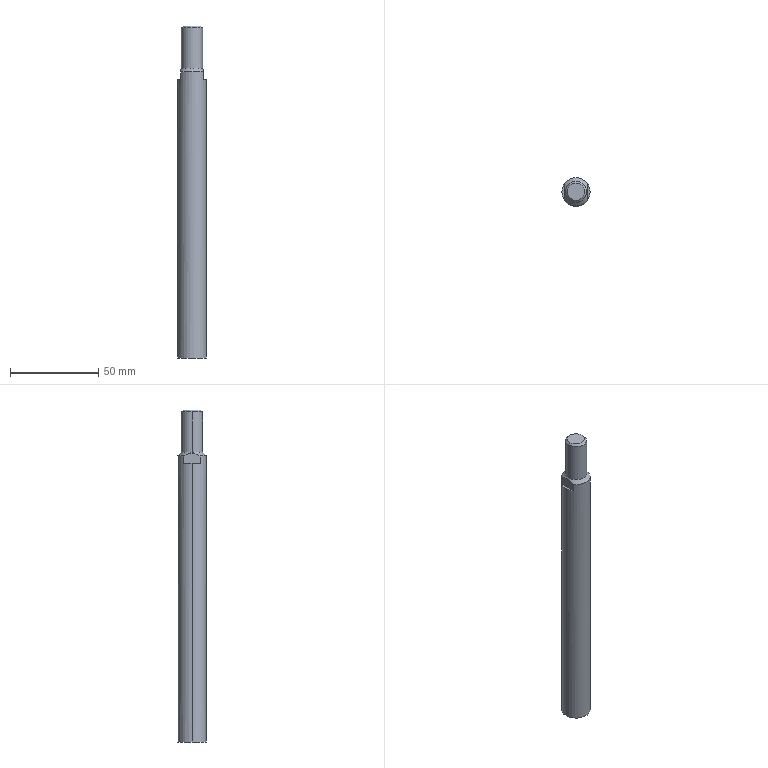Part | STEP file | fA_CP95SB40-150 (0)1 | 1 solid | 14 faces | box 16 x 16 x 188 mm | volume 35479 mm3 | plane 6 | cylinder 4 | cone 4 | commonest cylinder face diameters 12 x2 16 x2
STEP:
#1=CARTESIAN_POINT('',(0.,0.,0.));
#2=DIRECTION('',(0.,0.,1.));
#3=DIRECTION('',(1.,0.,0.));
#4=AXIS2_PLACEMENT_3D('',#1,#2,#3);
#5=CARTESIAN_POINT('',(8.,0.,-134.));
#6=VERTEX_POINT('',#5);
#7=CARTESIAN_POINT('',(-8.,0.,-134.));
#8=VERTEX_POINT('',#7);
#9=CARTESIAN_POINT('',(0.,0.,-134.));
#10=DIRECTION('',(0.,0.,1.));
#11=DIRECTION('',(1.,0.,0.));
#12=AXIS2_PLACEMENT_3D('',#9,#10,#11);
#13=CIRCLE('',#12,8.);
#14=CARTESIAN_POINT('',(0.,0.,28.));
#15=DIRECTION('',(0.,0.,1.));
#16=DIRECTION('',(1.,0.,0.));
#17=AXIS2_PLACEMENT_3D('',#14,#15,#16);
#18=CYLINDRICAL_SURFACE('',#17,8.);
#19=CARTESIAN_POINT('',(0.,-162.));
#20=DIRECTION('',(1.,0.));
#21=VECTOR('',#20,1.);
#22=LINE('',#19,#21);
#23=(GEOMETRIC_REPRESENTATION_CONTEXT(2)PARAMETRIC_REPRESENTATION_CONTEXT()REPRESENTATION_CONTEXT('',''));
#24=DEFINITIONAL_REPRESENTATION('',(#22),#23);
#25=PCURVE('',#18,#24);
#26=CARTESIAN_POINT('',(8.096,8.,-134.));
#27=DIRECTION('',(0.,0.,-1.));
#28=DIRECTION('',(-1.,0.,0.));
#29=AXIS2_PLACEMENT_3D('',#26,#27,#28);
#30=PLANE('',#29);
#31=CARTESIAN_POINT('',(0.096,-8.));
#32=CARTESIAN_POINT('',(0.096,5.856));
#33=CARTESIAN_POINT('',(12.096,-1.072));
#34=CARTESIAN_POINT('',(24.096,-8.));
#35=CARTESIAN_POINT('',(12.096,-14.928));
#36=CARTESIAN_POINT('',(0.096,-21.856));
#37=CARTESIAN_POINT('',(0.096,-8.));
#38=(BOUNDED_CURVE()B_SPLINE_CURVE(2,(#31,#32,#33,#34,#35,#36,#37),.UNSPECIFIED.,.T.,.F.)B_SPLINE_CURVE_WITH_KNOTS((1,2,2,2,2,1),(-2.094,0.,2.094,4.189,6.283,8.378),.UNSPECIFIED.)CURVE()GEOMETRIC_REPRESENTATION_ITEM()RATIONAL_B_SPLINE_CURVE((1.,0.5,1.,0.5,1.,0.5,1.))REPRESENTATION_ITEM(''));
#39=(GEOMETRIC_REPRESENTATION_CONTEXT(2)PARAMETRIC_REPRESENTATION_CONTEXT()REPRESENTATION_CONTEXT('',''));
#40=DEFINITIONAL_REPRESENTATION('',(#38),#39);
#41=PCURVE('',#30,#40);
#42=SURFACE_CURVE('',#13,(#25,#41),.PCURVE_S1.);
#43=EDGE_CURVE('',#6,#8,#42,.T.);
#44=ORIENTED_EDGE('',*,*,#43,.T.);
#45=CARTESIAN_POINT('',(-8.,0.,23.5));
#46=VERTEX_POINT('',#45);
#47=CARTESIAN_POINT('',(-8.,0.,28.));
#48=DIRECTION('',(0.,0.,1.));
#49=VECTOR('',#48,1.);
#50=LINE('',#47,#49);
#51=CARTESIAN_POINT('',(3.142,0.));
#52=DIRECTION('',(0.,1.));
#53=VECTOR('',#52,1.);
#54=LINE('',#51,#53);
#55=(GEOMETRIC_REPRESENTATION_CONTEXT(2)PARAMETRIC_REPRESENTATION_CONTEXT()REPRESENTATION_CONTEXT('',''));
#56=DEFINITIONAL_REPRESENTATION('',(#54),#55);
#57=PCURVE('',#18,#56);
#58=CARTESIAN_POINT('',(0.,0.,28.));
#59=DIRECTION('',(0.,0.,1.));
#60=DIRECTION('',(1.,0.,0.));
#61=AXIS2_PLACEMENT_3D('',#58,#59,#60);
#62=CYLINDRICAL_SURFACE('',#61,8.);
#63=CARTESIAN_POINT('',(3.142,0.));
#64=DIRECTION('',(0.,1.));
#65=VECTOR('',#64,1.);
#66=LINE('',#63,#65);
#67=(GEOMETRIC_REPRESENTATION_CONTEXT(2)PARAMETRIC_REPRESENTATION_CONTEXT()REPRESENTATION_CONTEXT('',''));
#68=DEFINITIONAL_REPRESENTATION('',(#66),#67);
#69=PCURVE('',#62,#68);
#70=SURFACE_CURVE('',#50,(#57,#69),.PCURVE_S1.);
#71=EDGE_CURVE('',#8,#46,#70,.T.);
#72=ORIENTED_EDGE('',*,*,#71,.T.);
#73=CARTESIAN_POINT('',(-6.5,4.664,23.5));
#74=VERTEX_POINT('',#73);
#75=CARTESIAN_POINT('',(0.,0.,23.5));
#76=DIRECTION('',(0.,0.,-1.));
#77=DIRECTION('',(1.,0.,0.));
#78=AXIS2_PLACEMENT_3D('',#75,#76,#77);
#79=CIRCLE('',#78,8.);
#80=CARTESIAN_POINT('',(6.283,-4.5));
#81=DIRECTION('',(-1.,0.));
#82=VECTOR('',#81,1.);
#83=LINE('',#80,#82);
#84=(GEOMETRIC_REPRESENTATION_CONTEXT(2)PARAMETRIC_REPRESENTATION_CONTEXT()REPRESENTATION_CONTEXT('',''));
#85=DEFINITIONAL_REPRESENTATION('',(#83),#84);
#86=PCURVE('',#18,#85);
#87=CARTESIAN_POINT('',(-8.009,-4.72,23.5));
#88=DIRECTION('',(0.,0.,1.));
#89=DIRECTION('',(1.,0.,0.));
#90=AXIS2_PLACEMENT_3D('',#87,#88,#89);
#91=PLANE('',#90);
#92=CARTESIAN_POINT('',(16.009,4.72));
#93=CARTESIAN_POINT('',(16.009,-9.137));
#94=CARTESIAN_POINT('',(4.009,-2.209));
#95=CARTESIAN_POINT('',(-7.991,4.72));
#96=CARTESIAN_POINT('',(4.009,11.648));
#97=CARTESIAN_POINT('',(16.009,18.576));
#98=CARTESIAN_POINT('',(16.009,4.72));
#99=(BOUNDED_CURVE()B_SPLINE_CURVE(2,(#92,#93,#94,#95,#96,#97,#98),.UNSPECIFIED.,.T.,.F.)B_SPLINE_CURVE_WITH_KNOTS((1,2,2,2,2,1),(-2.094,0.,2.094,4.189,6.283,8.378),.UNSPECIFIED.)CURVE()GEOMETRIC_REPRESENTATION_ITEM()RATIONAL_B_SPLINE_CURVE((1.,0.5,1.,0.5,1.,0.5,1.))REPRESENTATION_ITEM(''));
#100=(GEOMETRIC_REPRESENTATION_CONTEXT(2)PARAMETRIC_REPRESENTATION_CONTEXT()REPRESENTATION_CONTEXT('',''));
#101=DEFINITIONAL_REPRESENTATION('',(#99),#100);
#102=PCURVE('',#91,#101);
#103=SURFACE_CURVE('',#79,(#86,#102),.PCURVE_S1.);
#104=EDGE_CURVE('',#46,#74,#103,.T.);
#105=ORIENTED_EDGE('',*,*,#104,.T.);
#106=CARTESIAN_POINT('',(-6.5,4.664,28.));
#107=VERTEX_POINT('',#106);
#108=CARTESIAN_POINT('',(-6.5,4.664,28.));
#109=DIRECTION('',(0.,0.,1.));
#110=VECTOR('',#109,1.);
#111=LINE('',#108,#110);
#112=CARTESIAN_POINT('',(2.519,0.));
#113=DIRECTION('',(0.,1.));
#114=VECTOR('',#113,1.);
#115=LINE('',#112,#114);
#116=(GEOMETRIC_REPRESENTATION_CONTEXT(2)PARAMETRIC_REPRESENTATION_CONTEXT()REPRESENTATION_CONTEXT('',''));
#117=DEFINITIONAL_REPRESENTATION('',(#115),#116);
#118=PCURVE('',#18,#117);
#119=CARTESIAN_POINT('',(-6.5,-4.664,29.536));
#120=DIRECTION('',(-1.,0.,0.));
#121=DIRECTION('',(0.,0.,1.));
#122=AXIS2_PLACEMENT_3D('',#119,#120,#121);
#123=PLANE('',#122);
#124=CARTESIAN_POINT('',(-1.536,9.327));
#125=DIRECTION('',(1.,0.));
#126=VECTOR('',#125,1.);
#127=LINE('',#124,#126);
#128=(GEOMETRIC_REPRESENTATION_CONTEXT(2)PARAMETRIC_REPRESENTATION_CONTEXT()REPRESENTATION_CONTEXT('',''));
#129=DEFINITIONAL_REPRESENTATION('',(#127),#128);
#130=PCURVE('',#123,#129);
#131=SURFACE_CURVE('',#111,(#118,#130),.PCURVE_S1.);
#132=EDGE_CURVE('',#74,#107,#131,.T.);
#133=ORIENTED_EDGE('',*,*,#132,.T.);
#134=CARTESIAN_POINT('',(6.5,4.664,28.));
#135=VERTEX_POINT('',#134);
#136=CARTESIAN_POINT('',(0.,0.,28.));
#137=DIRECTION('',(0.,0.,-1.));
#138=DIRECTION('',(1.,0.,0.));
#139=AXIS2_PLACEMENT_3D('',#136,#137,#138);
#140=CIRCLE('',#139,8.);
#141=CARTESIAN_POINT('',(6.283,0.));
#142=DIRECTION('',(-1.,0.));
#143=VECTOR('',#142,1.);
#144=LINE('',#141,#143);
#145=(GEOMETRIC_REPRESENTATION_CONTEXT(2)PARAMETRIC_REPRESENTATION_CONTEXT()REPRESENTATION_CONTEXT('',''));
#146=DEFINITIONAL_REPRESENTATION('',(#144),#145);
#147=PCURVE('',#18,#146);
#148=CARTESIAN_POINT('',(0.,0.,28.));
#149=DIRECTION('',(0.,0.,-1.));
#150=DIRECTION('',(-1.,0.,0.));
#151=AXIS2_PLACEMENT_3D('',#148,#149,#150);
#152=CONICAL_SURFACE('',#151,8.,0.7854);
#153=CARTESIAN_POINT('',(-3.142,0.));
#154=DIRECTION('',(1.,0.));
#155=VECTOR('',#154,1.);
#156=LINE('',#153,#155);
#157=(GEOMETRIC_REPRESENTATION_CONTEXT(2)PARAMETRIC_REPRESENTATION_CONTEXT()REPRESENTATION_CONTEXT('',''));
#158=DEFINITIONAL_REPRESENTATION('',(#156),#157);
#159=PCURVE('',#152,#158);
#160=SURFACE_CURVE('',#140,(#147,#159),.PCURVE_S1.);
#161=EDGE_CURVE('',#107,#135,#160,.T.);
#162=ORIENTED_EDGE('',*,*,#161,.T.);
#163=CARTESIAN_POINT('',(6.5,4.664,23.5));
#164=VERTEX_POINT('',#163);
#165=CARTESIAN_POINT('',(6.5,4.664,28.));
#166=DIRECTION('',(0.,0.,-1.));
#167=VECTOR('',#166,1.);
#168=LINE('',#165,#167);
#169=CARTESIAN_POINT('',(0.6224,0.));
#170=DIRECTION('',(0.,-1.));
#171=VECTOR('',#170,1.);
#172=LINE('',#169,#171);
#173=(GEOMETRIC_REPRESENTATION_CONTEXT(2)PARAMETRIC_REPRESENTATION_CONTEXT()REPRESENTATION_CONTEXT('',''));
#174=DEFINITIONAL_REPRESENTATION('',(#172),#173);
#175=PCURVE('',#18,#174);
#176=CARTESIAN_POINT('',(6.5,4.664,29.536));
#177=DIRECTION('',(1.,0.,0.));
#178=DIRECTION('',(0.,0.,-1.));
#179=AXIS2_PLACEMENT_3D('',#176,#177,#178);
#180=PLANE('',#179);
#181=CARTESIAN_POINT('',(1.536,0.));
#182=DIRECTION('',(1.,0.));
#183=VECTOR('',#182,1.);
#184=LINE('',#181,#183);
#185=(GEOMETRIC_REPRESENTATION_CONTEXT(2)PARAMETRIC_REPRESENTATION_CONTEXT()REPRESENTATION_CONTEXT('',''));
#186=DEFINITIONAL_REPRESENTATION('',(#184),#185);
#187=PCURVE('',#180,#186);
#188=SURFACE_CURVE('',#168,(#175,#187),.PCURVE_S1.);
#189=EDGE_CURVE('',#135,#164,#188,.T.);
#190=ORIENTED_EDGE('',*,*,#189,.T.);
#191=CARTESIAN_POINT('',(8.,0.,23.5));
#192=VERTEX_POINT('',#191);
#193=CARTESIAN_POINT('',(0.,0.,23.5));
#194=DIRECTION('',(0.,0.,-1.));
#195=DIRECTION('',(1.,0.,0.));
#196=AXIS2_PLACEMENT_3D('',#193,#194,#195);
#197=CIRCLE('',#196,8.);
#198=CARTESIAN_POINT('',(6.283,-4.5));
#199=DIRECTION('',(-1.,0.));
#200=VECTOR('',#199,1.);
#201=LINE('',#198,#200);
#202=(GEOMETRIC_REPRESENTATION_CONTEXT(2)PARAMETRIC_REPRESENTATION_CONTEXT()REPRESENTATION_CONTEXT('',''));
#203=DEFINITIONAL_REPRESENTATION('',(#201),#202);
#204=PCURVE('',#18,#203);
#205=CARTESIAN_POINT('',(6.5,-4.72,23.5));
#206=DIRECTION('',(0.,0.,1.));
#207=DIRECTION('',(1.,0.,0.));
#208=AXIS2_PLACEMENT_3D('',#205,#206,#207);
#209=PLANE('',#208);
#210=CARTESIAN_POINT('',(1.5,4.72));
#211=CARTESIAN_POINT('',(1.5,-9.137));
#212=CARTESIAN_POINT('',(-10.5,-2.209));
#213=CARTESIAN_POINT('',(-22.5,4.72));
#214=CARTESIAN_POINT('',(-10.5,11.648));
#215=CARTESIAN_POINT('',(1.5,18.576));
#216=CARTESIAN_POINT('',(1.5,4.72));
#217=(BOUNDED_CURVE()B_SPLINE_CURVE(2,(#210,#211,#212,#213,#214,#215,#216),.UNSPECIFIED.,.T.,.F.)B_SPLINE_CURVE_WITH_KNOTS((1,2,2,2,2,1),(-2.094,0.,2.094,4.189,6.283,8.378),.UNSPECIFIED.)CURVE()GEOMETRIC_REPRESENTATION_ITEM()RATIONAL_B_SPLINE_CURVE((1.,0.5,1.,0.5,1.,0.5,1.))REPRESENTATION_ITEM(''));
#218=(GEOMETRIC_REPRESENTATION_CONTEXT(2)PARAMETRIC_REPRESENTATION_CONTEXT()REPRESENTATION_CONTEXT('',''));
#219=DEFINITIONAL_REPRESENTATION('',(#217),#218);
#220=PCURVE('',#209,#219);
#221=SURFACE_CURVE('',#197,(#204,#220),.PCURVE_S1.);
#222=EDGE_CURVE('',#164,#192,#221,.T.);
#223=ORIENTED_EDGE('',*,*,#222,.T.);
#224=CARTESIAN_POINT('',(8.,0.,28.));
#225=DIRECTION('',(0.,0.,1.));
#226=VECTOR('',#225,1.);
#227=LINE('',#224,#226);
#228=CARTESIAN_POINT('',(0.,0.));
#229=DIRECTION('',(0.,1.));
#230=VECTOR('',#229,1.);
#231=LINE('',#228,#230);
#232=(GEOMETRIC_REPRESENTATION_CONTEXT(2)PARAMETRIC_REPRESENTATION_CONTEXT()REPRESENTATION_CONTEXT('',''));
#233=DEFINITIONAL_REPRESENTATION('',(#231),#232);
#234=PCURVE('',#18,#233);
#235=CARTESIAN_POINT('',(6.283,0.));
#236=DIRECTION('',(0.,1.));
#237=VECTOR('',#236,1.);
#238=LINE('',#235,#237);
#239=(GEOMETRIC_REPRESENTATION_CONTEXT(2)PARAMETRIC_REPRESENTATION_CONTEXT()REPRESENTATION_CONTEXT('',''));
#240=DEFINITIONAL_REPRESENTATION('',(#238),#239);
#241=PCURVE('',#62,#240);
#242=SURFACE_CURVE('',#227,(#234,#241),.PCURVE_S1.);
#243=EDGE_CURVE('',#6,#192,#242,.T.);
#244=ORIENTED_EDGE('',*,*,#243,.F.);
#245=EDGE_LOOP('',(#44,#72,#105,#133,#162,#190,#223,#244));
#246=FACE_BOUND('',#245,.T.);
#247=ADVANCED_FACE('',(#246),#18,.T.);
#248=CARTESIAN_POINT('',(-6.,0.,30.));
#249=VERTEX_POINT('',#248);
#250=CARTESIAN_POINT('',(6.,0.,30.));
#251=VERTEX_POINT('',#250);
#252=CARTESIAN_POINT('',(0.,0.,30.));
#253=DIRECTION('',(0.,0.,-1.));
#254=DIRECTION('',(-1.,0.,0.));
#255=AXIS2_PLACEMENT_3D('',#252,#253,#254);
#256=CIRCLE('',#255,6.);
#257=CARTESIAN_POINT('',(0.,-2.));
#258=DIRECTION('',(1.,0.));
#259=VECTOR('',#258,1.);
#260=LINE('',#257,#259);
#261=(GEOMETRIC_REPRESENTATION_CONTEXT(2)PARAMETRIC_REPRESENTATION_CONTEXT()REPRESENTATION_CONTEXT('',''));
#262=DEFINITIONAL_REPRESENTATION('',(#260),#261);
#263=PCURVE('',#152,#262);
#264=CARTESIAN_POINT('',(0.,0.,52.926));
#265=DIRECTION('',(0.,0.,1.));
#266=DIRECTION('',(1.,0.,0.));
#267=AXIS2_PLACEMENT_3D('',#264,#265,#266);
#268=CYLINDRICAL_SURFACE('',#267,6.);
#269=CARTESIAN_POINT('',(3.142,-22.927));
#270=DIRECTION('',(-1.,0.));
#271=VECTOR('',#270,1.);
#272=LINE('',#269,#271);
#273=(GEOMETRIC_REPRESENTATION_CONTEXT(2)PARAMETRIC_REPRESENTATION_CONTEXT()REPRESENTATION_CONTEXT('',''));
#274=DEFINITIONAL_REPRESENTATION('',(#272),#273);
#275=PCURVE('',#268,#274);
#276=SURFACE_CURVE('',#256,(#263,#275),.PCURVE_S1.);
#277=EDGE_CURVE('',#249,#251,#276,.T.);
#278=ORIENTED_EDGE('',*,*,#277,.T.);
#279=CARTESIAN_POINT('',(6.5,0.,29.5));
#280=VERTEX_POINT('',#279);
#281=CARTESIAN_POINT('',(8.,0.,28.));
#282=DIRECTION('',(0.7071,0.,-0.7071));
#283=VECTOR('',#282,1.);
#284=LINE('',#281,#283);
#285=CARTESIAN_POINT('',(3.142,0.));
#286=DIRECTION('',(0.,1.));
#287=VECTOR('',#286,1.);
#288=LINE('',#285,#287);
#289=(GEOMETRIC_REPRESENTATION_CONTEXT(2)PARAMETRIC_REPRESENTATION_CONTEXT()REPRESENTATION_CONTEXT('',''));
#290=DEFINITIONAL_REPRESENTATION('',(#288),#289);
#291=PCURVE('',#152,#290);
#292=CARTESIAN_POINT('',(0.,0.,28.));
#293=DIRECTION('',(0.,0.,-1.));
#294=DIRECTION('',(-1.,0.,0.));
#295=AXIS2_PLACEMENT_3D('',#292,#293,#294);
#296=CONICAL_SURFACE('',#295,8.,0.7854);
#297=CARTESIAN_POINT('',(3.142,0.));
#298=DIRECTION('',(0.,1.));
#299=VECTOR('',#298,1.);
#300=LINE('',#297,#299);
#301=(GEOMETRIC_REPRESENTATION_CONTEXT(2)PARAMETRIC_REPRESENTATION_CONTEXT()REPRESENTATION_CONTEXT('',''));
#302=DEFINITIONAL_REPRESENTATION('',(#300),#301);
#303=PCURVE('',#296,#302);
#304=SURFACE_CURVE('',#284,(#291,#303),.PCURVE_S1.);
#305=EDGE_CURVE('',#251,#280,#304,.T.);
#306=ORIENTED_EDGE('',*,*,#305,.T.);
#307=CARTESIAN_POINT('',(6.5,4.664,28.));
#308=CARTESIAN_POINT('',(6.5,3.948,28.417));
#309=CARTESIAN_POINT('',(6.5,3.212,28.786));
#310=CARTESIAN_POINT('',(6.5,2.044,29.196));
#311=CARTESIAN_POINT('',(6.5,1.641,29.308));
#312=CARTESIAN_POINT('',(6.5,0.8281,29.46));
#313=CARTESIAN_POINT('',(6.5,0.4168,29.5));
#314=CARTESIAN_POINT('',(6.5,0.,29.5));
#315=B_SPLINE_CURVE_WITH_KNOTS('',3,(#307,#308,#309,#310,#311,#312,#313,#314),.UNSPECIFIED.,.F.,.F.,(4,2,2,4),(-0.004927,-0.002464,-0.001232,0.),.UNSPECIFIED.);
#316=CARTESIAN_POINT('',(2.519,0.));
#317=CARTESIAN_POINT('',(2.526,-0.03792));
#318=CARTESIAN_POINT('',(2.539,-0.1129));
#319=CARTESIAN_POINT('',(2.56,-0.2228));
#320=CARTESIAN_POINT('',(2.582,-0.3299));
#321=CARTESIAN_POINT('',(2.604,-0.434));
#322=CARTESIAN_POINT('',(2.627,-0.5348));
#323=CARTESIAN_POINT('',(2.651,-0.6323));
#324=CARTESIAN_POINT('',(2.676,-0.7261));
#325=CARTESIAN_POINT('',(2.701,-0.816));
#326=CARTESIAN_POINT('',(2.728,-0.9018));
#327=CARTESIAN_POINT('',(2.755,-0.9833));
#328=CARTESIAN_POINT('',(2.783,-1.06));
#329=CARTESIAN_POINT('',(2.812,-1.132));
#330=CARTESIAN_POINT('',(2.842,-1.199));
#331=CARTESIAN_POINT('',(2.873,-1.26));
#332=CARTESIAN_POINT('',(2.905,-1.315));
#333=CARTESIAN_POINT('',(2.937,-1.363));
#334=CARTESIAN_POINT('',(2.97,-1.405));
#335=CARTESIAN_POINT('',(3.004,-1.439));
#336=CARTESIAN_POINT('',(3.038,-1.466));
#337=CARTESIAN_POINT('',(3.072,-1.486));
#338=CARTESIAN_POINT('',(3.107,-1.497));
#339=CARTESIAN_POINT('',(3.13,-1.5));
#340=CARTESIAN_POINT('',(3.142,-1.5));
#341=B_SPLINE_CURVE_WITH_KNOTS('',3,(#316,#317,#318,#319,#320,#321,#322,#323,#324,#325,#326,#327,#328,#329,#330,#331,#332,#333,#334,#335,#336,#337,#338,#339,#340),.UNSPECIFIED.,.F.,.F.,(4,1,1,1,1,1,1,1,1,1,1,1,1,1,1,1,1,1,1,1,1,1,4),(-0.004927,-0.004703,-0.004479,-0.004255,-0.004031,-0.003807,-0.003583,-0.003359,-0.003136,-0.002912,-0.002688,-0.002464,-0.00224,-0.002016,-0.001792,-0.001568,-0.001344,-0.00112,-0.0008959,-0.0006719,-0.0004479,-0.000224,0.),.UNSPECIFIED.);
#342=(GEOMETRIC_REPRESENTATION_CONTEXT(2)PARAMETRIC_REPRESENTATION_CONTEXT()REPRESENTATION_CONTEXT('',''));
#343=DEFINITIONAL_REPRESENTATION('',(#341),#342);
#344=PCURVE('',#152,#343);
#345=CARTESIAN_POINT('',(1.536,0.));
#346=CARTESIAN_POINT('',(1.119,-0.7155));
#347=CARTESIAN_POINT('',(0.7496,-1.452));
#348=CARTESIAN_POINT('',(0.3402,-2.619));
#349=CARTESIAN_POINT('',(0.2281,-3.022));
#350=CARTESIAN_POINT('',(0.07635,-3.836));
#351=CARTESIAN_POINT('',(0.036,-4.247));
#352=CARTESIAN_POINT('',(0.036,-4.664));
#353=B_SPLINE_CURVE_WITH_KNOTS('',3,(#345,#346,#347,#348,#349,#350,#351,#352),.UNSPECIFIED.,.F.,.F.,(4,2,2,4),(-0.004927,-0.002464,-0.001232,0.),.UNSPECIFIED.);
#354=(GEOMETRIC_REPRESENTATION_CONTEXT(2)PARAMETRIC_REPRESENTATION_CONTEXT()REPRESENTATION_CONTEXT('',''));
#355=DEFINITIONAL_REPRESENTATION('',(#353),#354);
#356=PCURVE('',#180,#355);
#357=SURFACE_CURVE('',#315,(#344,#356),.PCURVE_S1.);
#358=EDGE_CURVE('',#135,#280,#357,.T.);
#359=ORIENTED_EDGE('',*,*,#358,.F.);
#360=ORIENTED_EDGE('',*,*,#161,.F.);
#361=CARTESIAN_POINT('',(-6.5,0.,29.5));
#362=VERTEX_POINT('',#361);
#363=CARTESIAN_POINT('',(-6.5,4.664,28.));
#364=CARTESIAN_POINT('',(-6.5,3.948,28.417));
#365=CARTESIAN_POINT('',(-6.5,3.212,28.786));
#366=CARTESIAN_POINT('',(-6.5,2.044,29.196));
#367=CARTESIAN_POINT('',(-6.5,1.641,29.308));
#368=CARTESIAN_POINT('',(-6.5,0.8281,29.46));
#369=CARTESIAN_POINT('',(-6.5,0.4168,29.5));
#370=CARTESIAN_POINT('',(-6.5,0.,29.5));
#371=B_SPLINE_CURVE_WITH_KNOTS('',3,(#363,#364,#365,#366,#367,#368,#369,#370),.UNSPECIFIED.,.F.,.F.,(4,2,2,4),(0.,0.002468,0.003701,0.004935),.UNSPECIFIED.);
#372=CARTESIAN_POINT('',(0.6224,0.));
#373=CARTESIAN_POINT('',(0.6158,-0.03792));
#374=CARTESIAN_POINT('',(0.6023,-0.1129));
#375=CARTESIAN_POINT('',(0.5815,-0.2228));
#376=CARTESIAN_POINT('',(0.5599,-0.3299));
#377=CARTESIAN_POINT('',(0.5376,-0.434));
#378=CARTESIAN_POINT('',(0.5145,-0.5348));
#379=CARTESIAN_POINT('',(0.4906,-0.6323));
#380=CARTESIAN_POINT('',(0.4659,-0.7261));
#381=CARTESIAN_POINT('',(0.4403,-0.816));
#382=CARTESIAN_POINT('',(0.4139,-0.9018));
#383=CARTESIAN_POINT('',(0.3866,-0.9833));
#384=CARTESIAN_POINT('',(0.3584,-1.06));
#385=CARTESIAN_POINT('',(0.3293,-1.132));
#386=CARTESIAN_POINT('',(0.2992,-1.199));
#387=CARTESIAN_POINT('',(0.2683,-1.26));
#388=CARTESIAN_POINT('',(0.2366,-1.315));
#389=CARTESIAN_POINT('',(0.2042,-1.363));
#390=CARTESIAN_POINT('',(0.1713,-1.405));
#391=CARTESIAN_POINT('',(0.1378,-1.439));
#392=CARTESIAN_POINT('',(0.1039,-1.466));
#393=CARTESIAN_POINT('',(0.06956,-1.486));
#394=CARTESIAN_POINT('',(0.03492,-1.497));
#395=CARTESIAN_POINT('',(0.01166,-1.5));
#396=CARTESIAN_POINT('',(0.,-1.5));
#397=B_SPLINE_CURVE_WITH_KNOTS('',3,(#372,#373,#374,#375,#376,#377,#378,#379,#380,#381,#382,#383,#384,#385,#386,#387,#388,#389,#390,#391,#392,#393,#394,#395,#396),.UNSPECIFIED.,.F.,.F.,(4,1,1,1,1,1,1,1,1,1,1,1,1,1,1,1,1,1,1,1,1,1,4),(0.,0.0002243,0.0004487,0.000673,0.0008973,0.001122,0.001346,0.00157,0.001795,0.002019,0.002243,0.002468,0.002692,0.002916,0.003141,0.003365,0.003589,0.003814,0.004038,0.004262,0.004487,0.004711,0.004935),.QUASI_UNIFORM_KNOTS.);
#398=(GEOMETRIC_REPRESENTATION_CONTEXT(2)PARAMETRIC_REPRESENTATION_CONTEXT()REPRESENTATION_CONTEXT('',''));
#399=DEFINITIONAL_REPRESENTATION('',(#397),#398);
#400=PCURVE('',#152,#399);
#401=CARTESIAN_POINT('',(-1.536,9.327));
#402=CARTESIAN_POINT('',(-1.119,8.612));
#403=CARTESIAN_POINT('',(-0.7496,7.876));
#404=CARTESIAN_POINT('',(-0.3402,6.708));
#405=CARTESIAN_POINT('',(-0.2281,6.305));
#406=CARTESIAN_POINT('',(-0.07635,5.492));
#407=CARTESIAN_POINT('',(-0.036,5.08));
#408=CARTESIAN_POINT('',(-0.036,4.664));
#409=B_SPLINE_CURVE_WITH_KNOTS('',3,(#401,#402,#403,#404,#405,#406,#407,#408),.UNSPECIFIED.,.F.,.F.,(4,2,2,4),(0.,0.002468,0.003701,0.004935),.UNSPECIFIED.);
#410=(GEOMETRIC_REPRESENTATION_CONTEXT(2)PARAMETRIC_REPRESENTATION_CONTEXT()REPRESENTATION_CONTEXT('',''));
#411=DEFINITIONAL_REPRESENTATION('',(#409),#410);
#412=PCURVE('',#123,#411);
#413=SURFACE_CURVE('',#371,(#400,#412),.PCURVE_S1.);
#414=EDGE_CURVE('',#107,#362,#413,.T.);
#415=ORIENTED_EDGE('',*,*,#414,.T.);
#416=CARTESIAN_POINT('',(-8.,0.,28.));
#417=DIRECTION('',(-0.7071,0.,-0.7071));
#418=VECTOR('',#417,1.);
#419=LINE('',#416,#418);
#420=CARTESIAN_POINT('',(0.,0.));
#421=DIRECTION('',(0.,1.));
#422=VECTOR('',#421,1.);
#423=LINE('',#420,#422);
#424=(GEOMETRIC_REPRESENTATION_CONTEXT(2)PARAMETRIC_REPRESENTATION_CONTEXT()REPRESENTATION_CONTEXT('',''));
#425=DEFINITIONAL_REPRESENTATION('',(#423),#424);
#426=PCURVE('',#152,#425);
#427=CARTESIAN_POINT('',(6.283,0.));
#428=DIRECTION('',(0.,1.));
#429=VECTOR('',#428,1.);
#430=LINE('',#427,#429);
#431=(GEOMETRIC_REPRESENTATION_CONTEXT(2)PARAMETRIC_REPRESENTATION_CONTEXT()REPRESENTATION_CONTEXT('',''));
#432=DEFINITIONAL_REPRESENTATION('',(#430),#431);
#433=PCURVE('',#296,#432);
#434=SURFACE_CURVE('',#419,(#426,#433),.PCURVE_S1.);
#435=EDGE_CURVE('',#249,#362,#434,.T.);
#436=ORIENTED_EDGE('',*,*,#435,.F.);
#437=EDGE_LOOP('',(#278,#306,#359,#360,#415,#436));
#438=FACE_BOUND('',#437,.T.);
#439=ADVANCED_FACE('',(#438),#152,.T.);
#440=ORIENTED_EDGE('',*,*,#277,.F.);
#441=CARTESIAN_POINT('',(-6.,0.,52.926));
#442=VERTEX_POINT('',#441);
#443=CARTESIAN_POINT('',(-6.,0.,52.926));
#444=DIRECTION('',(0.,0.,1.));
#445=VECTOR('',#444,1.);
#446=LINE('',#443,#445);
#447=CARTESIAN_POINT('',(3.142,0.));
#448=DIRECTION('',(0.,1.));
#449=VECTOR('',#448,1.);
#450=LINE('',#447,#449);
#451=(GEOMETRIC_REPRESENTATION_CONTEXT(2)PARAMETRIC_REPRESENTATION_CONTEXT()REPRESENTATION_CONTEXT('',''));
#452=DEFINITIONAL_REPRESENTATION('',(#450),#451);
#453=PCURVE('',#268,#452);
#454=CARTESIAN_POINT('',(0.,0.,52.926));
#455=DIRECTION('',(0.,0.,1.));
#456=DIRECTION('',(1.,0.,0.));
#457=AXIS2_PLACEMENT_3D('',#454,#455,#456);
#458=CYLINDRICAL_SURFACE('',#457,6.);
#459=CARTESIAN_POINT('',(3.142,0.));
#460=DIRECTION('',(0.,1.));
#461=VECTOR('',#460,1.);
#462=LINE('',#459,#461);
#463=(GEOMETRIC_REPRESENTATION_CONTEXT(2)PARAMETRIC_REPRESENTATION_CONTEXT()REPRESENTATION_CONTEXT('',''));
#464=DEFINITIONAL_REPRESENTATION('',(#462),#463);
#465=PCURVE('',#458,#464);
#466=SURFACE_CURVE('',#446,(#453,#465),.PCURVE_S1.);
#467=EDGE_CURVE('',#249,#442,#466,.T.);
#468=ORIENTED_EDGE('',*,*,#467,.T.);
#469=CARTESIAN_POINT('',(6.,0.,52.926));
#470=VERTEX_POINT('',#469);
#471=CARTESIAN_POINT('',(0.,0.,52.926));
#472=DIRECTION('',(0.,0.,-1.));
#473=DIRECTION('',(1.,0.,0.));
#474=AXIS2_PLACEMENT_3D('',#471,#472,#473);
#475=CIRCLE('',#474,6.);
#476=CARTESIAN_POINT('',(6.283,0.));
#477=DIRECTION('',(-1.,0.));
#478=VECTOR('',#477,1.);
#479=LINE('',#476,#478);
#480=(GEOMETRIC_REPRESENTATION_CONTEXT(2)PARAMETRIC_REPRESENTATION_CONTEXT()REPRESENTATION_CONTEXT('',''));
#481=DEFINITIONAL_REPRESENTATION('',(#479),#480);
#482=PCURVE('',#268,#481);
#483=CARTESIAN_POINT('',(0.,0.,52.926));
#484=DIRECTION('',(0.,0.,-1.));
#485=DIRECTION('',(-1.,0.,0.));
#486=AXIS2_PLACEMENT_3D('',#483,#484,#485);
#487=CONICAL_SURFACE('',#486,6.,0.7854);
#488=CARTESIAN_POINT('',(-3.142,0.));
#489=DIRECTION('',(1.,0.));
#490=VECTOR('',#489,1.);
#491=LINE('',#488,#490);
#492=(GEOMETRIC_REPRESENTATION_CONTEXT(2)PARAMETRIC_REPRESENTATION_CONTEXT()REPRESENTATION_CONTEXT('',''));
#493=DEFINITIONAL_REPRESENTATION('',(#491),#492);
#494=PCURVE('',#487,#493);
#495=SURFACE_CURVE('',#475,(#482,#494),.PCURVE_S1.);
#496=EDGE_CURVE('',#442,#470,#495,.T.);
#497=ORIENTED_EDGE('',*,*,#496,.T.);
#498=CARTESIAN_POINT('',(6.,0.,52.926));
#499=DIRECTION('',(0.,0.,1.));
#500=VECTOR('',#499,1.);
#501=LINE('',#498,#500);
#502=CARTESIAN_POINT('',(0.,0.));
#503=DIRECTION('',(0.,1.));
#504=VECTOR('',#503,1.);
#505=LINE('',#502,#504);
#506=(GEOMETRIC_REPRESENTATION_CONTEXT(2)PARAMETRIC_REPRESENTATION_CONTEXT()REPRESENTATION_CONTEXT('',''));
#507=DEFINITIONAL_REPRESENTATION('',(#505),#506);
#508=PCURVE('',#268,#507);
#509=CARTESIAN_POINT('',(6.283,0.));
#510=DIRECTION('',(0.,1.));
#511=VECTOR('',#510,1.);
#512=LINE('',#509,#511);
#513=(GEOMETRIC_REPRESENTATION_CONTEXT(2)PARAMETRIC_REPRESENTATION_CONTEXT()REPRESENTATION_CONTEXT('',''));
#514=DEFINITIONAL_REPRESENTATION('',(#512),#513);
#515=PCURVE('',#458,#514);
#516=SURFACE_CURVE('',#501,(#508,#515),.PCURVE_S1.);
#517=EDGE_CURVE('',#251,#470,#516,.T.);
#518=ORIENTED_EDGE('',*,*,#517,.F.);
#519=EDGE_LOOP('',(#440,#468,#497,#518));
#520=FACE_BOUND('',#519,.T.);
#521=ADVANCED_FACE('',(#520),#268,.T.);
#522=CARTESIAN_POINT('',(-4.926,0.,54.));
#523=VERTEX_POINT('',#522);
#524=CARTESIAN_POINT('',(4.926,0.,54.));
#525=VERTEX_POINT('',#524);
#526=CARTESIAN_POINT('',(0.,0.,54.));
#527=DIRECTION('',(0.,0.,-1.));
#528=DIRECTION('',(-1.,0.,0.));
#529=AXIS2_PLACEMENT_3D('',#526,#527,#528);
#530=CIRCLE('',#529,4.926);
#531=CARTESIAN_POINT('',(0.,-1.074));
#532=DIRECTION('',(1.,0.));
#533=VECTOR('',#532,1.);
#534=LINE('',#531,#533);
#535=(GEOMETRIC_REPRESENTATION_CONTEXT(2)PARAMETRIC_REPRESENTATION_CONTEXT()REPRESENTATION_CONTEXT('',''));
#536=DEFINITIONAL_REPRESENTATION('',(#534),#535);
#537=PCURVE('',#487,#536);
#538=CARTESIAN_POINT('',(4.986,-4.926,54.));
#539=DIRECTION('',(0.,0.,1.));
#540=DIRECTION('',(1.,0.,0.));
#541=AXIS2_PLACEMENT_3D('',#538,#539,#540);
#542=PLANE('',#541);
#543=CARTESIAN_POINT('',(-9.912,4.926));
#544=CARTESIAN_POINT('',(-9.912,13.459));
#545=CARTESIAN_POINT('',(-2.522,9.193));
#546=CARTESIAN_POINT('',(4.867,4.926));
#547=CARTESIAN_POINT('',(-2.522,0.66));
#548=CARTESIAN_POINT('',(-9.912,-3.606));
#549=CARTESIAN_POINT('',(-9.912,4.926));
#550=(BOUNDED_CURVE()B_SPLINE_CURVE(2,(#543,#544,#545,#546,#547,#548,#549),.UNSPECIFIED.,.T.,.F.)B_SPLINE_CURVE_WITH_KNOTS((1,2,2,2,2,1),(-2.094,0.,2.094,4.189,6.283,8.378),.UNSPECIFIED.)CURVE()GEOMETRIC_REPRESENTATION_ITEM()RATIONAL_B_SPLINE_CURVE((1.,0.5,1.,0.5,1.,0.5,1.))REPRESENTATION_ITEM(''));
#551=(GEOMETRIC_REPRESENTATION_CONTEXT(2)PARAMETRIC_REPRESENTATION_CONTEXT()REPRESENTATION_CONTEXT('',''));
#552=DEFINITIONAL_REPRESENTATION('',(#550),#551);
#553=PCURVE('',#542,#552);
#554=SURFACE_CURVE('',#530,(#537,#553),.PCURVE_S1.);
#555=EDGE_CURVE('',#523,#525,#554,.T.);
#556=ORIENTED_EDGE('',*,*,#555,.T.);
#557=CARTESIAN_POINT('',(6.,0.,52.926));
#558=DIRECTION('',(0.7071,0.,-0.7071));
#559=VECTOR('',#558,1.);
#560=LINE('',#557,#559);
#561=CARTESIAN_POINT('',(3.142,0.));
#562=DIRECTION('',(0.,1.));
#563=VECTOR('',#562,1.);
#564=LINE('',#561,#563);
#565=(GEOMETRIC_REPRESENTATION_CONTEXT(2)PARAMETRIC_REPRESENTATION_CONTEXT()REPRESENTATION_CONTEXT('',''));
#566=DEFINITIONAL_REPRESENTATION('',(#564),#565);
#567=PCURVE('',#487,#566);
#568=CARTESIAN_POINT('',(0.,0.,52.926));
#569=DIRECTION('',(0.,0.,-1.));
#570=DIRECTION('',(-1.,0.,0.));
#571=AXIS2_PLACEMENT_3D('',#568,#569,#570);
#572=CONICAL_SURFACE('',#571,6.,0.7854);
#573=CARTESIAN_POINT('',(3.142,0.));
#574=DIRECTION('',(0.,1.));
#575=VECTOR('',#574,1.);
#576=LINE('',#573,#575);
#577=(GEOMETRIC_REPRESENTATION_CONTEXT(2)PARAMETRIC_REPRESENTATION_CONTEXT()REPRESENTATION_CONTEXT('',''));
#578=DEFINITIONAL_REPRESENTATION('',(#576),#577);
#579=PCURVE('',#572,#578);
#580=SURFACE_CURVE('',#560,(#567,#579),.PCURVE_S1.);
#581=EDGE_CURVE('',#525,#470,#580,.T.);
#582=ORIENTED_EDGE('',*,*,#581,.T.);
#583=ORIENTED_EDGE('',*,*,#496,.F.);
#584=CARTESIAN_POINT('',(-6.,0.,52.926));
#585=DIRECTION('',(-0.7071,0.,-0.7071));
#586=VECTOR('',#585,1.);
#587=LINE('',#584,#586);
#588=CARTESIAN_POINT('',(0.,0.));
#589=DIRECTION('',(0.,1.));
#590=VECTOR('',#589,1.);
#591=LINE('',#588,#590);
#592=(GEOMETRIC_REPRESENTATION_CONTEXT(2)PARAMETRIC_REPRESENTATION_CONTEXT()REPRESENTATION_CONTEXT('',''));
#593=DEFINITIONAL_REPRESENTATION('',(#591),#592);
#594=PCURVE('',#487,#593);
#595=CARTESIAN_POINT('',(6.283,0.));
#596=DIRECTION('',(0.,1.));
#597=VECTOR('',#596,1.);
#598=LINE('',#595,#597);
#599=(GEOMETRIC_REPRESENTATION_CONTEXT(2)PARAMETRIC_REPRESENTATION_CONTEXT()REPRESENTATION_CONTEXT('',''));
#600=DEFINITIONAL_REPRESENTATION('',(#598),#599);
#601=PCURVE('',#572,#600);
#602=SURFACE_CURVE('',#587,(#594,#601),.PCURVE_S1.);
#603=EDGE_CURVE('',#523,#442,#602,.T.);
#604=ORIENTED_EDGE('',*,*,#603,.F.);
#605=EDGE_LOOP('',(#556,#582,#583,#604));
#606=FACE_BOUND('',#605,.T.);
#607=ADVANCED_FACE('',(#606),#487,.T.);
#608=ORIENTED_EDGE('',*,*,#71,.F.);
#609=CARTESIAN_POINT('',(0.,0.,-134.));
#610=DIRECTION('',(0.,0.,1.));
#611=DIRECTION('',(1.,0.,0.));
#612=AXIS2_PLACEMENT_3D('',#609,#610,#611);
#613=CIRCLE('',#612,8.);
#614=CARTESIAN_POINT('',(0.,-162.));
#615=DIRECTION('',(1.,0.));
#616=VECTOR('',#615,1.);
#617=LINE('',#614,#616);
#618=(GEOMETRIC_REPRESENTATION_CONTEXT(2)PARAMETRIC_REPRESENTATION_CONTEXT()REPRESENTATION_CONTEXT('',''));
#619=DEFINITIONAL_REPRESENTATION('',(#617),#618);
#620=PCURVE('',#62,#619);
#621=CARTESIAN_POINT('',(0.096,-8.));
#622=CARTESIAN_POINT('',(0.096,5.856));
#623=CARTESIAN_POINT('',(12.096,-1.072));
#624=CARTESIAN_POINT('',(24.096,-8.));
#625=CARTESIAN_POINT('',(12.096,-14.928));
#626=CARTESIAN_POINT('',(0.096,-21.856));
#627=CARTESIAN_POINT('',(0.096,-8.));
#628=(BOUNDED_CURVE()B_SPLINE_CURVE(2,(#621,#622,#623,#624,#625,#626,#627),.UNSPECIFIED.,.T.,.F.)B_SPLINE_CURVE_WITH_KNOTS((1,2,2,2,2,1),(-2.094,0.,2.094,4.189,6.283,8.378),.UNSPECIFIED.)CURVE()GEOMETRIC_REPRESENTATION_ITEM()RATIONAL_B_SPLINE_CURVE((1.,0.5,1.,0.5,1.,0.5,1.))REPRESENTATION_ITEM(''));
#629=(GEOMETRIC_REPRESENTATION_CONTEXT(2)PARAMETRIC_REPRESENTATION_CONTEXT()REPRESENTATION_CONTEXT('',''));
#630=DEFINITIONAL_REPRESENTATION('',(#628),#629);
#631=PCURVE('',#30,#630);
#632=SURFACE_CURVE('',#613,(#620,#631),.PCURVE_S1.);
#633=EDGE_CURVE('',#8,#6,#632,.T.);
#634=ORIENTED_EDGE('',*,*,#633,.T.);
#635=ORIENTED_EDGE('',*,*,#243,.T.);
#636=CARTESIAN_POINT('',(6.5,-4.664,23.5));
#637=VERTEX_POINT('',#636);
#638=CARTESIAN_POINT('',(0.,0.,23.5));
#639=DIRECTION('',(0.,0.,-1.));
#640=DIRECTION('',(1.,0.,0.));
#641=AXIS2_PLACEMENT_3D('',#638,#639,#640);
#642=CIRCLE('',#641,8.);
#643=CARTESIAN_POINT('',(6.283,-4.5));
#644=DIRECTION('',(-1.,0.));
#645=VECTOR('',#644,1.);
#646=LINE('',#643,#645);
#647=(GEOMETRIC_REPRESENTATION_CONTEXT(2)PARAMETRIC_REPRESENTATION_CONTEXT()REPRESENTATION_CONTEXT('',''));
#648=DEFINITIONAL_REPRESENTATION('',(#646),#647);
#649=PCURVE('',#62,#648);
#650=CARTESIAN_POINT('',(1.5,4.72));
#651=CARTESIAN_POINT('',(1.5,-9.137));
#652=CARTESIAN_POINT('',(-10.5,-2.209));
#653=CARTESIAN_POINT('',(-22.5,4.72));
#654=CARTESIAN_POINT('',(-10.5,11.648));
#655=CARTESIAN_POINT('',(1.5,18.576));
#656=CARTESIAN_POINT('',(1.5,4.72));
#657=(BOUNDED_CURVE()B_SPLINE_CURVE(2,(#650,#651,#652,#653,#654,#655,#656),.UNSPECIFIED.,.T.,.F.)B_SPLINE_CURVE_WITH_KNOTS((1,2,2,2,2,1),(-2.094,0.,2.094,4.189,6.283,8.378),.UNSPECIFIED.)CURVE()GEOMETRIC_REPRESENTATION_ITEM()RATIONAL_B_SPLINE_CURVE((1.,0.5,1.,0.5,1.,0.5,1.))REPRESENTATION_ITEM(''));
#658=(GEOMETRIC_REPRESENTATION_CONTEXT(2)PARAMETRIC_REPRESENTATION_CONTEXT()REPRESENTATION_CONTEXT('',''));
#659=DEFINITIONAL_REPRESENTATION('',(#657),#658);
#660=PCURVE('',#209,#659);
#661=SURFACE_CURVE('',#642,(#649,#660),.PCURVE_S1.);
#662=EDGE_CURVE('',#192,#637,#661,.T.);
#663=ORIENTED_EDGE('',*,*,#662,.T.);
#664=CARTESIAN_POINT('',(6.5,-4.664,28.));
#665=VERTEX_POINT('',#664);
#666=CARTESIAN_POINT('',(6.5,-4.664,28.));
#667=DIRECTION('',(0.,0.,1.));
#668=VECTOR('',#667,1.);
#669=LINE('',#666,#668);
#670=CARTESIAN_POINT('',(5.661,0.));
#671=DIRECTION('',(0.,1.));
#672=VECTOR('',#671,1.);
#673=LINE('',#670,#672);
#674=(GEOMETRIC_REPRESENTATION_CONTEXT(2)PARAMETRIC_REPRESENTATION_CONTEXT()REPRESENTATION_CONTEXT('',''));
#675=DEFINITIONAL_REPRESENTATION('',(#673),#674);
#676=PCURVE('',#62,#675);
#677=CARTESIAN_POINT('',(1.536,-9.327));
#678=DIRECTION('',(-1.,0.));
#679=VECTOR('',#678,1.);
#680=LINE('',#677,#679);
#681=(GEOMETRIC_REPRESENTATION_CONTEXT(2)PARAMETRIC_REPRESENTATION_CONTEXT()REPRESENTATION_CONTEXT('',''));
#682=DEFINITIONAL_REPRESENTATION('',(#680),#681);
#683=PCURVE('',#180,#682);
#684=SURFACE_CURVE('',#669,(#676,#683),.PCURVE_S1.);
#685=EDGE_CURVE('',#637,#665,#684,.T.);
#686=ORIENTED_EDGE('',*,*,#685,.T.);
#687=CARTESIAN_POINT('',(-6.5,-4.664,28.));
#688=VERTEX_POINT('',#687);
#689=CARTESIAN_POINT('',(0.,0.,28.));
#690=DIRECTION('',(0.,0.,-1.));
#691=DIRECTION('',(1.,0.,0.));
#692=AXIS2_PLACEMENT_3D('',#689,#690,#691);
#693=CIRCLE('',#692,8.);
#694=CARTESIAN_POINT('',(6.283,0.));
#695=DIRECTION('',(-1.,0.));
#696=VECTOR('',#695,1.);
#697=LINE('',#694,#696);
#698=(GEOMETRIC_REPRESENTATION_CONTEXT(2)PARAMETRIC_REPRESENTATION_CONTEXT()REPRESENTATION_CONTEXT('',''));
#699=DEFINITIONAL_REPRESENTATION('',(#697),#698);
#700=PCURVE('',#62,#699);
#701=CARTESIAN_POINT('',(3.142,0.));
#702=DIRECTION('',(1.,0.));
#703=VECTOR('',#702,1.);
#704=LINE('',#701,#703);
#705=(GEOMETRIC_REPRESENTATION_CONTEXT(2)PARAMETRIC_REPRESENTATION_CONTEXT()REPRESENTATION_CONTEXT('',''));
#706=DEFINITIONAL_REPRESENTATION('',(#704),#705);
#707=PCURVE('',#296,#706);
#708=SURFACE_CURVE('',#693,(#700,#707),.PCURVE_S1.);
#709=EDGE_CURVE('',#665,#688,#708,.T.);
#710=ORIENTED_EDGE('',*,*,#709,.T.);
#711=CARTESIAN_POINT('',(-6.5,-4.664,23.5));
#712=VERTEX_POINT('',#711);
#713=CARTESIAN_POINT('',(-6.5,-4.664,28.));
#714=DIRECTION('',(0.,0.,-1.));
#715=VECTOR('',#714,1.);
#716=LINE('',#713,#715);
#717=CARTESIAN_POINT('',(3.764,0.));
#718=DIRECTION('',(0.,-1.));
#719=VECTOR('',#718,1.);
#720=LINE('',#717,#719);
#721=(GEOMETRIC_REPRESENTATION_CONTEXT(2)PARAMETRIC_REPRESENTATION_CONTEXT()REPRESENTATION_CONTEXT('',''));
#722=DEFINITIONAL_REPRESENTATION('',(#720),#721);
#723=PCURVE('',#62,#722);
#724=CARTESIAN_POINT('',(-1.536,0.));
#725=DIRECTION('',(-1.,0.));
#726=VECTOR('',#725,1.);
#727=LINE('',#724,#726);
#728=(GEOMETRIC_REPRESENTATION_CONTEXT(2)PARAMETRIC_REPRESENTATION_CONTEXT()REPRESENTATION_CONTEXT('',''));
#729=DEFINITIONAL_REPRESENTATION('',(#727),#728);
#730=PCURVE('',#123,#729);
#731=SURFACE_CURVE('',#716,(#723,#730),.PCURVE_S1.);
#732=EDGE_CURVE('',#688,#712,#731,.T.);
#733=ORIENTED_EDGE('',*,*,#732,.T.);
#734=CARTESIAN_POINT('',(0.,0.,23.5));
#735=DIRECTION('',(0.,0.,-1.));
#736=DIRECTION('',(1.,0.,0.));
#737=AXIS2_PLACEMENT_3D('',#734,#735,#736);
#738=CIRCLE('',#737,8.);
#739=CARTESIAN_POINT('',(6.283,-4.5));
#740=DIRECTION('',(-1.,0.));
#741=VECTOR('',#740,1.);
#742=LINE('',#739,#741);
#743=(GEOMETRIC_REPRESENTATION_CONTEXT(2)PARAMETRIC_REPRESENTATION_CONTEXT()REPRESENTATION_CONTEXT('',''));
#744=DEFINITIONAL_REPRESENTATION('',(#742),#743);
#745=PCURVE('',#62,#744);
#746=CARTESIAN_POINT('',(16.009,4.72));
#747=CARTESIAN_POINT('',(16.009,-9.137));
#748=CARTESIAN_POINT('',(4.009,-2.209));
#749=CARTESIAN_POINT('',(-7.991,4.72));
#750=CARTESIAN_POINT('',(4.009,11.648));
#751=CARTESIAN_POINT('',(16.009,18.576));
#752=CARTESIAN_POINT('',(16.009,4.72));
#753=(BOUNDED_CURVE()B_SPLINE_CURVE(2,(#746,#747,#748,#749,#750,#751,#752),.UNSPECIFIED.,.T.,.F.)B_SPLINE_CURVE_WITH_KNOTS((1,2,2,2,2,1),(-2.094,0.,2.094,4.189,6.283,8.378),.UNSPECIFIED.)CURVE()GEOMETRIC_REPRESENTATION_ITEM()RATIONAL_B_SPLINE_CURVE((1.,0.5,1.,0.5,1.,0.5,1.))REPRESENTATION_ITEM(''));
#754=(GEOMETRIC_REPRESENTATION_CONTEXT(2)PARAMETRIC_REPRESENTATION_CONTEXT()REPRESENTATION_CONTEXT('',''));
#755=DEFINITIONAL_REPRESENTATION('',(#753),#754);
#756=PCURVE('',#91,#755);
#757=SURFACE_CURVE('',#738,(#745,#756),.PCURVE_S1.);
#758=EDGE_CURVE('',#712,#46,#757,.T.);
#759=ORIENTED_EDGE('',*,*,#758,.T.);
#760=EDGE_LOOP('',(#608,#634,#635,#663,#686,#710,#733,#759));
#761=FACE_BOUND('',#760,.T.);
#762=ADVANCED_FACE('',(#761),#62,.T.);
#763=CARTESIAN_POINT('',(6.5,0.,23.5));
#764=DIRECTION('',(0.,-1.,0.));
#765=VECTOR('',#764,1.);
#766=LINE('',#763,#765);
#767=CARTESIAN_POINT('',(0.,4.72));
#768=DIRECTION('',(0.,-1.));
#769=VECTOR('',#768,1.);
#770=LINE('',#767,#769);
#771=(GEOMETRIC_REPRESENTATION_CONTEXT(2)PARAMETRIC_REPRESENTATION_CONTEXT()REPRESENTATION_CONTEXT('',''));
#772=DEFINITIONAL_REPRESENTATION('',(#770),#771);
#773=PCURVE('',#209,#772);
#774=CARTESIAN_POINT('',(6.036,-4.664));
#775=DIRECTION('',(0.,-1.));
#776=VECTOR('',#775,1.);
#777=LINE('',#774,#776);
#778=(GEOMETRIC_REPRESENTATION_CONTEXT(2)PARAMETRIC_REPRESENTATION_CONTEXT()REPRESENTATION_CONTEXT('',''));
#779=DEFINITIONAL_REPRESENTATION('',(#777),#778);
#780=PCURVE('',#180,#779);
#781=SURFACE_CURVE('',#766,(#773,#780),.PCURVE_S1.);
#782=EDGE_CURVE('',#164,#637,#781,.T.);
#783=ORIENTED_EDGE('',*,*,#782,.T.);
#784=ORIENTED_EDGE('',*,*,#662,.F.);
#785=ORIENTED_EDGE('',*,*,#222,.F.);
#786=EDGE_LOOP('',(#783,#784,#785));
#787=FACE_BOUND('',#786,.T.);
#788=ADVANCED_FACE('',(#787),#209,.T.);
#789=ORIENTED_EDGE('',*,*,#189,.F.);
#790=ORIENTED_EDGE('',*,*,#358,.T.);
#791=CARTESIAN_POINT('',(6.5,0.,29.5));
#792=CARTESIAN_POINT('',(6.5,-0.4169,29.5));
#793=CARTESIAN_POINT('',(6.5,-0.8268,29.46));
#794=CARTESIAN_POINT('',(6.5,-1.634,29.309));
#795=CARTESIAN_POINT('',(6.5,-2.033,29.199));
#796=CARTESIAN_POINT('',(6.5,-3.209,28.788));
#797=CARTESIAN_POINT('',(6.5,-3.947,28.418));
#798=CARTESIAN_POINT('',(6.5,-4.664,28.));
#799=B_SPLINE_CURVE_WITH_KNOTS('',3,(#791,#792,#793,#794,#795,#796,#797,#798),.UNSPECIFIED.,.F.,.F.,(4,2,2,4),(0.,0.001232,0.002464,0.004929),.UNSPECIFIED.);
#800=CARTESIAN_POINT('',(0.036,-4.664));
#801=CARTESIAN_POINT('',(0.036,-5.081));
#802=CARTESIAN_POINT('',(0.07635,-5.49));
#803=CARTESIAN_POINT('',(0.2266,-6.298));
#804=CARTESIAN_POINT('',(0.3367,-6.697));
#805=CARTESIAN_POINT('',(0.7477,-7.873));
#806=CARTESIAN_POINT('',(1.118,-8.611));
#807=CARTESIAN_POINT('',(1.536,-9.327));
#808=B_SPLINE_CURVE_WITH_KNOTS('',3,(#800,#801,#802,#803,#804,#805,#806,#807),.UNSPECIFIED.,.F.,.F.,(4,2,2,4),(0.,0.001232,0.002464,0.004929),.UNSPECIFIED.);
#809=(GEOMETRIC_REPRESENTATION_CONTEXT(2)PARAMETRIC_REPRESENTATION_CONTEXT()REPRESENTATION_CONTEXT('',''));
#810=DEFINITIONAL_REPRESENTATION('',(#808),#809);
#811=PCURVE('',#180,#810);
#812=CARTESIAN_POINT('',(3.142,-1.5));
#813=CARTESIAN_POINT('',(3.153,-1.5));
#814=CARTESIAN_POINT('',(3.177,-1.497));
#815=CARTESIAN_POINT('',(3.211,-1.486));
#816=CARTESIAN_POINT('',(3.245,-1.466));
#817=CARTESIAN_POINT('',(3.279,-1.439));
#818=CARTESIAN_POINT('',(3.312,-1.405));
#819=CARTESIAN_POINT('',(3.345,-1.364));
#820=CARTESIAN_POINT('',(3.377,-1.317));
#821=CARTESIAN_POINT('',(3.409,-1.262));
#822=CARTESIAN_POINT('',(3.44,-1.202));
#823=CARTESIAN_POINT('',(3.47,-1.135));
#824=CARTESIAN_POINT('',(3.499,-1.063));
#825=CARTESIAN_POINT('',(3.527,-0.9859));
#826=CARTESIAN_POINT('',(3.555,-0.9042));
#827=CARTESIAN_POINT('',(3.581,-0.818));
#828=CARTESIAN_POINT('',(3.607,-0.7278));
#829=CARTESIAN_POINT('',(3.632,-0.6337));
#830=CARTESIAN_POINT('',(3.656,-0.5359));
#831=CARTESIAN_POINT('',(3.679,-0.4348));
#832=CARTESIAN_POINT('',(3.701,-0.3305));
#833=CARTESIAN_POINT('',(3.723,-0.2232));
#834=CARTESIAN_POINT('',(3.744,-0.1131));
#835=CARTESIAN_POINT('',(3.757,-0.03796));
#836=CARTESIAN_POINT('',(3.764,0.));
#837=B_SPLINE_CURVE_WITH_KNOTS('',3,(#812,#813,#814,#815,#816,#817,#818,#819,#820,#821,#822,#823,#824,#825,#826,#827,#828,#829,#830,#831,#832,#833,#834,#835,#836),.UNSPECIFIED.,.F.,.F.,(4,1,1,1,1,1,1,1,1,1,1,1,1,1,1,1,1,1,1,1,1,1,4),(0.,0.000224,0.0004481,0.0006721,0.0008962,0.00112,0.001344,0.001568,0.001792,0.002016,0.00224,0.002464,0.002689,0.002913,0.003137,0.003361,0.003585,0.003809,0.004033,0.004257,0.004481,0.004705,0.004929),.QUASI_UNIFORM_KNOTS.);
#838=(GEOMETRIC_REPRESENTATION_CONTEXT(2)PARAMETRIC_REPRESENTATION_CONTEXT()REPRESENTATION_CONTEXT('',''));
#839=DEFINITIONAL_REPRESENTATION('',(#837),#838);
#840=PCURVE('',#296,#839);
#841=SURFACE_CURVE('',#799,(#811,#840),.PCURVE_S1.);
#842=EDGE_CURVE('',#280,#665,#841,.T.);
#843=ORIENTED_EDGE('',*,*,#842,.T.);
#844=ORIENTED_EDGE('',*,*,#685,.F.);
#845=ORIENTED_EDGE('',*,*,#782,.F.);
#846=EDGE_LOOP('',(#789,#790,#843,#844,#845));
#847=FACE_BOUND('',#846,.T.);
#848=ADVANCED_FACE('',(#847),#180,.T.);
#849=ORIENTED_EDGE('',*,*,#305,.F.);
#850=CARTESIAN_POINT('',(0.,0.,30.));
#851=DIRECTION('',(0.,0.,-1.));
#852=DIRECTION('',(-1.,0.,0.));
#853=AXIS2_PLACEMENT_3D('',#850,#851,#852);
#854=CIRCLE('',#853,6.);
#855=CARTESIAN_POINT('',(0.,-2.));
#856=DIRECTION('',(1.,0.));
#857=VECTOR('',#856,1.);
#858=LINE('',#855,#857);
#859=(GEOMETRIC_REPRESENTATION_CONTEXT(2)PARAMETRIC_REPRESENTATION_CONTEXT()REPRESENTATION_CONTEXT('',''));
#860=DEFINITIONAL_REPRESENTATION('',(#858),#859);
#861=PCURVE('',#296,#860);
#862=CARTESIAN_POINT('',(9.425,-22.927));
#863=DIRECTION('',(-1.,0.));
#864=VECTOR('',#863,1.);
#865=LINE('',#862,#864);
#866=(GEOMETRIC_REPRESENTATION_CONTEXT(2)PARAMETRIC_REPRESENTATION_CONTEXT()REPRESENTATION_CONTEXT('',''));
#867=DEFINITIONAL_REPRESENTATION('',(#865),#866);
#868=PCURVE('',#458,#867);
#869=SURFACE_CURVE('',#854,(#861,#868),.PCURVE_S1.);
#870=EDGE_CURVE('',#251,#249,#869,.T.);
#871=ORIENTED_EDGE('',*,*,#870,.T.);
#872=ORIENTED_EDGE('',*,*,#435,.T.);
#873=CARTESIAN_POINT('',(-6.5,0.,29.5));
#874=CARTESIAN_POINT('',(-6.5,-0.4169,29.5));
#875=CARTESIAN_POINT('',(-6.5,-0.8268,29.46));
#876=CARTESIAN_POINT('',(-6.5,-1.634,29.309));
#877=CARTESIAN_POINT('',(-6.5,-2.033,29.199));
#878=CARTESIAN_POINT('',(-6.5,-3.209,28.788));
#879=CARTESIAN_POINT('',(-6.5,-3.947,28.418));
#880=CARTESIAN_POINT('',(-6.5,-4.664,28.));
#881=B_SPLINE_CURVE_WITH_KNOTS('',3,(#873,#874,#875,#876,#877,#878,#879,#880),.UNSPECIFIED.,.F.,.F.,(4,2,2,4),(0.004935,0.006169,0.007404,0.009872),.UNSPECIFIED.);
#882=CARTESIAN_POINT('',(6.283,-1.5));
#883=CARTESIAN_POINT('',(6.272,-1.5));
#884=CARTESIAN_POINT('',(6.248,-1.497));
#885=CARTESIAN_POINT('',(6.214,-1.486));
#886=CARTESIAN_POINT('',(6.179,-1.466));
#887=CARTESIAN_POINT('',(6.146,-1.439));
#888=CARTESIAN_POINT('',(6.112,-1.405));
#889=CARTESIAN_POINT('',(6.08,-1.364));
#890=CARTESIAN_POINT('',(6.048,-1.317));
#891=CARTESIAN_POINT('',(6.016,-1.262));
#892=CARTESIAN_POINT('',(5.985,-1.202));
#893=CARTESIAN_POINT('',(5.955,-1.135));
#894=CARTESIAN_POINT('',(5.926,-1.063));
#895=CARTESIAN_POINT('',(5.898,-0.9859));
#896=CARTESIAN_POINT('',(5.87,-0.9042));
#897=CARTESIAN_POINT('',(5.843,-0.818));
#898=CARTESIAN_POINT('',(5.818,-0.7278));
#899=CARTESIAN_POINT('',(5.793,-0.6337));
#900=CARTESIAN_POINT('',(5.769,-0.5359));
#901=CARTESIAN_POINT('',(5.746,-0.4348));
#902=CARTESIAN_POINT('',(5.723,-0.3305));
#903=CARTESIAN_POINT('',(5.702,-0.2232));
#904=CARTESIAN_POINT('',(5.681,-0.1131));
#905=CARTESIAN_POINT('',(5.667,-0.03796));
#906=CARTESIAN_POINT('',(5.661,0.));
#907=B_SPLINE_CURVE_WITH_KNOTS('',3,(#882,#883,#884,#885,#886,#887,#888,#889,#890,#891,#892,#893,#894,#895,#896,#897,#898,#899,#900,#901,#902,#903,#904,#905,#906),.UNSPECIFIED.,.F.,.F.,(4,1,1,1,1,1,1,1,1,1,1,1,1,1,1,1,1,1,1,1,1,1,4),(0.004935,0.00516,0.005384,0.005608,0.005833,0.006057,0.006282,0.006506,0.00673,0.006955,0.007179,0.007404,0.007628,0.007853,0.008077,0.008301,0.008526,0.00875,0.008975,0.009199,0.009423,0.009648,0.009872),.QUASI_UNIFORM_KNOTS.);
#908=(GEOMETRIC_REPRESENTATION_CONTEXT(2)PARAMETRIC_REPRESENTATION_CONTEXT()REPRESENTATION_CONTEXT('',''));
#909=DEFINITIONAL_REPRESENTATION('',(#907),#908);
#910=PCURVE('',#296,#909);
#911=CARTESIAN_POINT('',(-0.036,4.664));
#912=CARTESIAN_POINT('',(-0.036,4.247));
#913=CARTESIAN_POINT('',(-0.07635,3.837));
#914=CARTESIAN_POINT('',(-0.2266,3.029));
#915=CARTESIAN_POINT('',(-0.3367,2.63));
#916=CARTESIAN_POINT('',(-0.7477,1.455));
#917=CARTESIAN_POINT('',(-1.118,0.7164));
#918=CARTESIAN_POINT('',(-1.536,0.));
#919=B_SPLINE_CURVE_WITH_KNOTS('',3,(#911,#912,#913,#914,#915,#916,#917,#918),.UNSPECIFIED.,.F.,.F.,(4,2,2,4),(0.004935,0.006169,0.007404,0.009872),.UNSPECIFIED.);
#920=(GEOMETRIC_REPRESENTATION_CONTEXT(2)PARAMETRIC_REPRESENTATION_CONTEXT()REPRESENTATION_CONTEXT('',''));
#921=DEFINITIONAL_REPRESENTATION('',(#919),#920);
#922=PCURVE('',#123,#921);
#923=SURFACE_CURVE('',#881,(#910,#922),.PCURVE_S1.);
#924=EDGE_CURVE('',#362,#688,#923,.T.);
#925=ORIENTED_EDGE('',*,*,#924,.T.);
#926=ORIENTED_EDGE('',*,*,#709,.F.);
#927=ORIENTED_EDGE('',*,*,#842,.F.);
#928=EDGE_LOOP('',(#849,#871,#872,#925,#926,#927));
#929=FACE_BOUND('',#928,.T.);
#930=ADVANCED_FACE('',(#929),#296,.T.);
#931=ORIENTED_EDGE('',*,*,#732,.F.);
#932=ORIENTED_EDGE('',*,*,#924,.F.);
#933=ORIENTED_EDGE('',*,*,#414,.F.);
#934=ORIENTED_EDGE('',*,*,#132,.F.);
#935=CARTESIAN_POINT('',(-6.5,-4.664,23.5));
#936=DIRECTION('',(0.,-1.,0.));
#937=VECTOR('',#936,1.);
#938=LINE('',#935,#937);
#939=CARTESIAN_POINT('',(-6.036,0.));
#940=DIRECTION('',(0.,-1.));
#941=VECTOR('',#940,1.);
#942=LINE('',#939,#941);
#943=(GEOMETRIC_REPRESENTATION_CONTEXT(2)PARAMETRIC_REPRESENTATION_CONTEXT()REPRESENTATION_CONTEXT('',''));
#944=DEFINITIONAL_REPRESENTATION('',(#942),#943);
#945=PCURVE('',#123,#944);
#946=CARTESIAN_POINT('',(1.509,0.05596));
#947=DIRECTION('',(0.,-1.));
#948=VECTOR('',#947,1.);
#949=LINE('',#946,#948);
#950=(GEOMETRIC_REPRESENTATION_CONTEXT(2)PARAMETRIC_REPRESENTATION_CONTEXT()REPRESENTATION_CONTEXT('',''));
#951=DEFINITIONAL_REPRESENTATION('',(#949),#950);
#952=PCURVE('',#91,#951);
#953=SURFACE_CURVE('',#938,(#945,#952),.PCURVE_S1.);
#954=EDGE_CURVE('',#74,#712,#953,.T.);
#955=ORIENTED_EDGE('',*,*,#954,.T.);
#956=EDGE_LOOP('',(#931,#932,#933,#934,#955));
#957=FACE_BOUND('',#956,.T.);
#958=ADVANCED_FACE('',(#957),#123,.T.);
#959=ORIENTED_EDGE('',*,*,#954,.F.);
#960=ORIENTED_EDGE('',*,*,#104,.F.);
#961=ORIENTED_EDGE('',*,*,#758,.F.);
#962=EDGE_LOOP('',(#959,#960,#961));
#963=FACE_BOUND('',#962,.T.);
#964=ADVANCED_FACE('',(#963),#91,.T.);
#965=ORIENTED_EDGE('',*,*,#43,.F.);
#966=ORIENTED_EDGE('',*,*,#633,.F.);
#967=EDGE_LOOP('',(#965,#966));
#968=FACE_BOUND('',#967,.T.);
#969=ADVANCED_FACE('',(#968),#30,.T.);
#970=ORIENTED_EDGE('',*,*,#467,.F.);
#971=ORIENTED_EDGE('',*,*,#870,.F.);
#972=ORIENTED_EDGE('',*,*,#517,.T.);
#973=CARTESIAN_POINT('',(0.,0.,52.926));
#974=DIRECTION('',(0.,0.,-1.));
#975=DIRECTION('',(1.,0.,0.));
#976=AXIS2_PLACEMENT_3D('',#973,#974,#975);
#977=CIRCLE('',#976,6.);
#978=CARTESIAN_POINT('',(6.283,0.));
#979=DIRECTION('',(-1.,0.));
#980=VECTOR('',#979,1.);
#981=LINE('',#978,#980);
#982=(GEOMETRIC_REPRESENTATION_CONTEXT(2)PARAMETRIC_REPRESENTATION_CONTEXT()REPRESENTATION_CONTEXT('',''));
#983=DEFINITIONAL_REPRESENTATION('',(#981),#982);
#984=PCURVE('',#458,#983);
#985=CARTESIAN_POINT('',(3.142,0.));
#986=DIRECTION('',(1.,0.));
#987=VECTOR('',#986,1.);
#988=LINE('',#985,#987);
#989=(GEOMETRIC_REPRESENTATION_CONTEXT(2)PARAMETRIC_REPRESENTATION_CONTEXT()REPRESENTATION_CONTEXT('',''));
#990=DEFINITIONAL_REPRESENTATION('',(#988),#989);
#991=PCURVE('',#572,#990);
#992=SURFACE_CURVE('',#977,(#984,#991),.PCURVE_S1.);
#993=EDGE_CURVE('',#470,#442,#992,.T.);
#994=ORIENTED_EDGE('',*,*,#993,.T.);
#995=EDGE_LOOP('',(#970,#971,#972,#994));
#996=FACE_BOUND('',#995,.T.);
#997=ADVANCED_FACE('',(#996),#458,.T.);
#998=ORIENTED_EDGE('',*,*,#581,.F.);
#999=CARTESIAN_POINT('',(0.,0.,54.));
#1000=DIRECTION('',(0.,0.,-1.));
#1001=DIRECTION('',(-1.,0.,0.));
#1002=AXIS2_PLACEMENT_3D('',#999,#1000,#1001);
#1003=CIRCLE('',#1002,4.926);
#1004=CARTESIAN_POINT('',(0.,-1.074));
#1005=DIRECTION('',(1.,0.));
#1006=VECTOR('',#1005,1.);
#1007=LINE('',#1004,#1006);
#1008=(GEOMETRIC_REPRESENTATION_CONTEXT(2)PARAMETRIC_REPRESENTATION_CONTEXT()REPRESENTATION_CONTEXT('',''));
#1009=DEFINITIONAL_REPRESENTATION('',(#1007),#1008);
#1010=PCURVE('',#572,#1009);
#1011=CARTESIAN_POINT('',(-9.912,4.926));
#1012=CARTESIAN_POINT('',(-9.912,13.459));
#1013=CARTESIAN_POINT('',(-2.522,9.193));
#1014=CARTESIAN_POINT('',(4.867,4.926));
#1015=CARTESIAN_POINT('',(-2.522,0.66));
#1016=CARTESIAN_POINT('',(-9.912,-3.606));
#1017=CARTESIAN_POINT('',(-9.912,4.926));
#1018=(BOUNDED_CURVE()B_SPLINE_CURVE(2,(#1011,#1012,#1013,#1014,#1015,#1016,#1017),.UNSPECIFIED.,.T.,.F.)B_SPLINE_CURVE_WITH_KNOTS((1,2,2,2,2,1),(-2.094,0.,2.094,4.189,6.283,8.378),.UNSPECIFIED.)CURVE()GEOMETRIC_REPRESENTATION_ITEM()RATIONAL_B_SPLINE_CURVE((1.,0.5,1.,0.5,1.,0.5,1.))REPRESENTATION_ITEM(''));
#1019=(GEOMETRIC_REPRESENTATION_CONTEXT(2)PARAMETRIC_REPRESENTATION_CONTEXT()REPRESENTATION_CONTEXT('',''));
#1020=DEFINITIONAL_REPRESENTATION('',(#1018),#1019);
#1021=PCURVE('',#542,#1020);
#1022=SURFACE_CURVE('',#1003,(#1010,#1021),.PCURVE_S1.);
#1023=EDGE_CURVE('',#525,#523,#1022,.T.);
#1024=ORIENTED_EDGE('',*,*,#1023,.T.);
#1025=ORIENTED_EDGE('',*,*,#603,.T.);
#1026=ORIENTED_EDGE('',*,*,#993,.F.);
#1027=EDGE_LOOP('',(#998,#1024,#1025,#1026));
#1028=FACE_BOUND('',#1027,.T.);
#1029=ADVANCED_FACE('',(#1028),#572,.T.);
#1030=ORIENTED_EDGE('',*,*,#555,.F.);
#1031=ORIENTED_EDGE('',*,*,#1023,.F.);
#1032=EDGE_LOOP('',(#1030,#1031));
#1033=FACE_BOUND('',#1032,.T.);
#1034=ADVANCED_FACE('',(#1033),#542,.T.);
#1035=CLOSED_SHELL('',(#247,#439,#521,#607,#762,#788,#848,#930,#958,#964,#969,#997,#1029,#1034));
#1036=MANIFOLD_SOLID_BREP('',#1035);
#1037=(LENGTH_UNIT()NAMED_UNIT(*)SI_UNIT(.MILLI.,.METRE.));
#1038=UNCERTAINTY_MEASURE_WITH_UNIT(LENGTH_MEASURE(0.0001),#1037,'','');
#1039=(NAMED_UNIT(*)PLANE_ANGLE_UNIT()SI_UNIT($,.RADIAN.));
#1040=(NAMED_UNIT(*)SI_UNIT($,.STERADIAN.)SOLID_ANGLE_UNIT());
#1041=(GEOMETRIC_REPRESENTATION_CONTEXT(3)GLOBAL_UNCERTAINTY_ASSIGNED_CONTEXT((#1038))GLOBAL_UNIT_ASSIGNED_CONTEXT((#1037,#1039,#1040))REPRESENTATION_CONTEXT('',''));
#1042=ADVANCED_BREP_SHAPE_REPRESENTATION('',(#4,#1036),#1041);